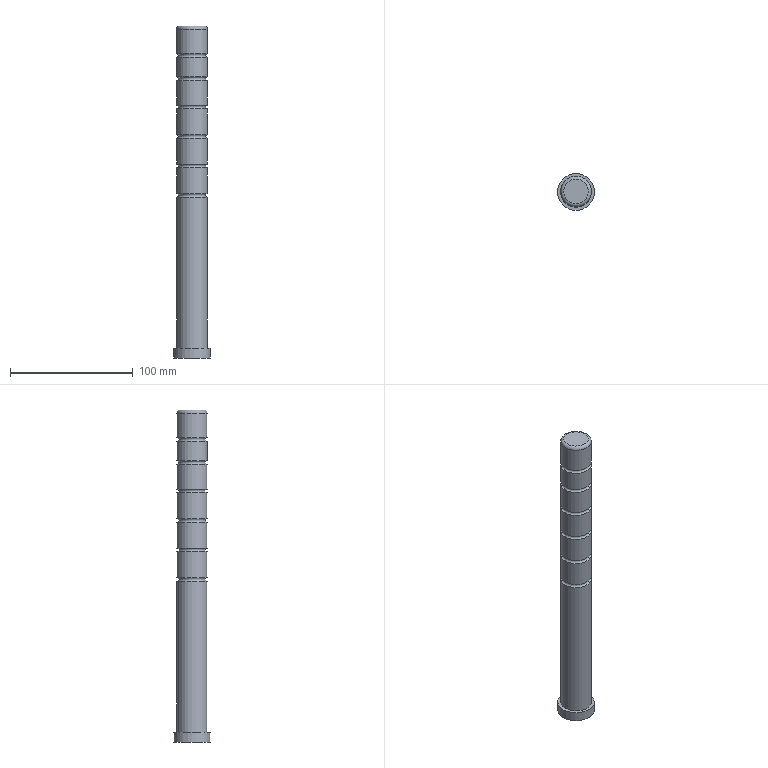Part | STEP file | solid 22 | 1 solid | 22 faces | box 30 x 30 x 270.5 mm | volume 130641 mm3 | cylinder 10 | torus 7 | plane 4 | cone 1 | commonest cylinder face diameters 25 x7 8.5 x1 10 x1 30 x1